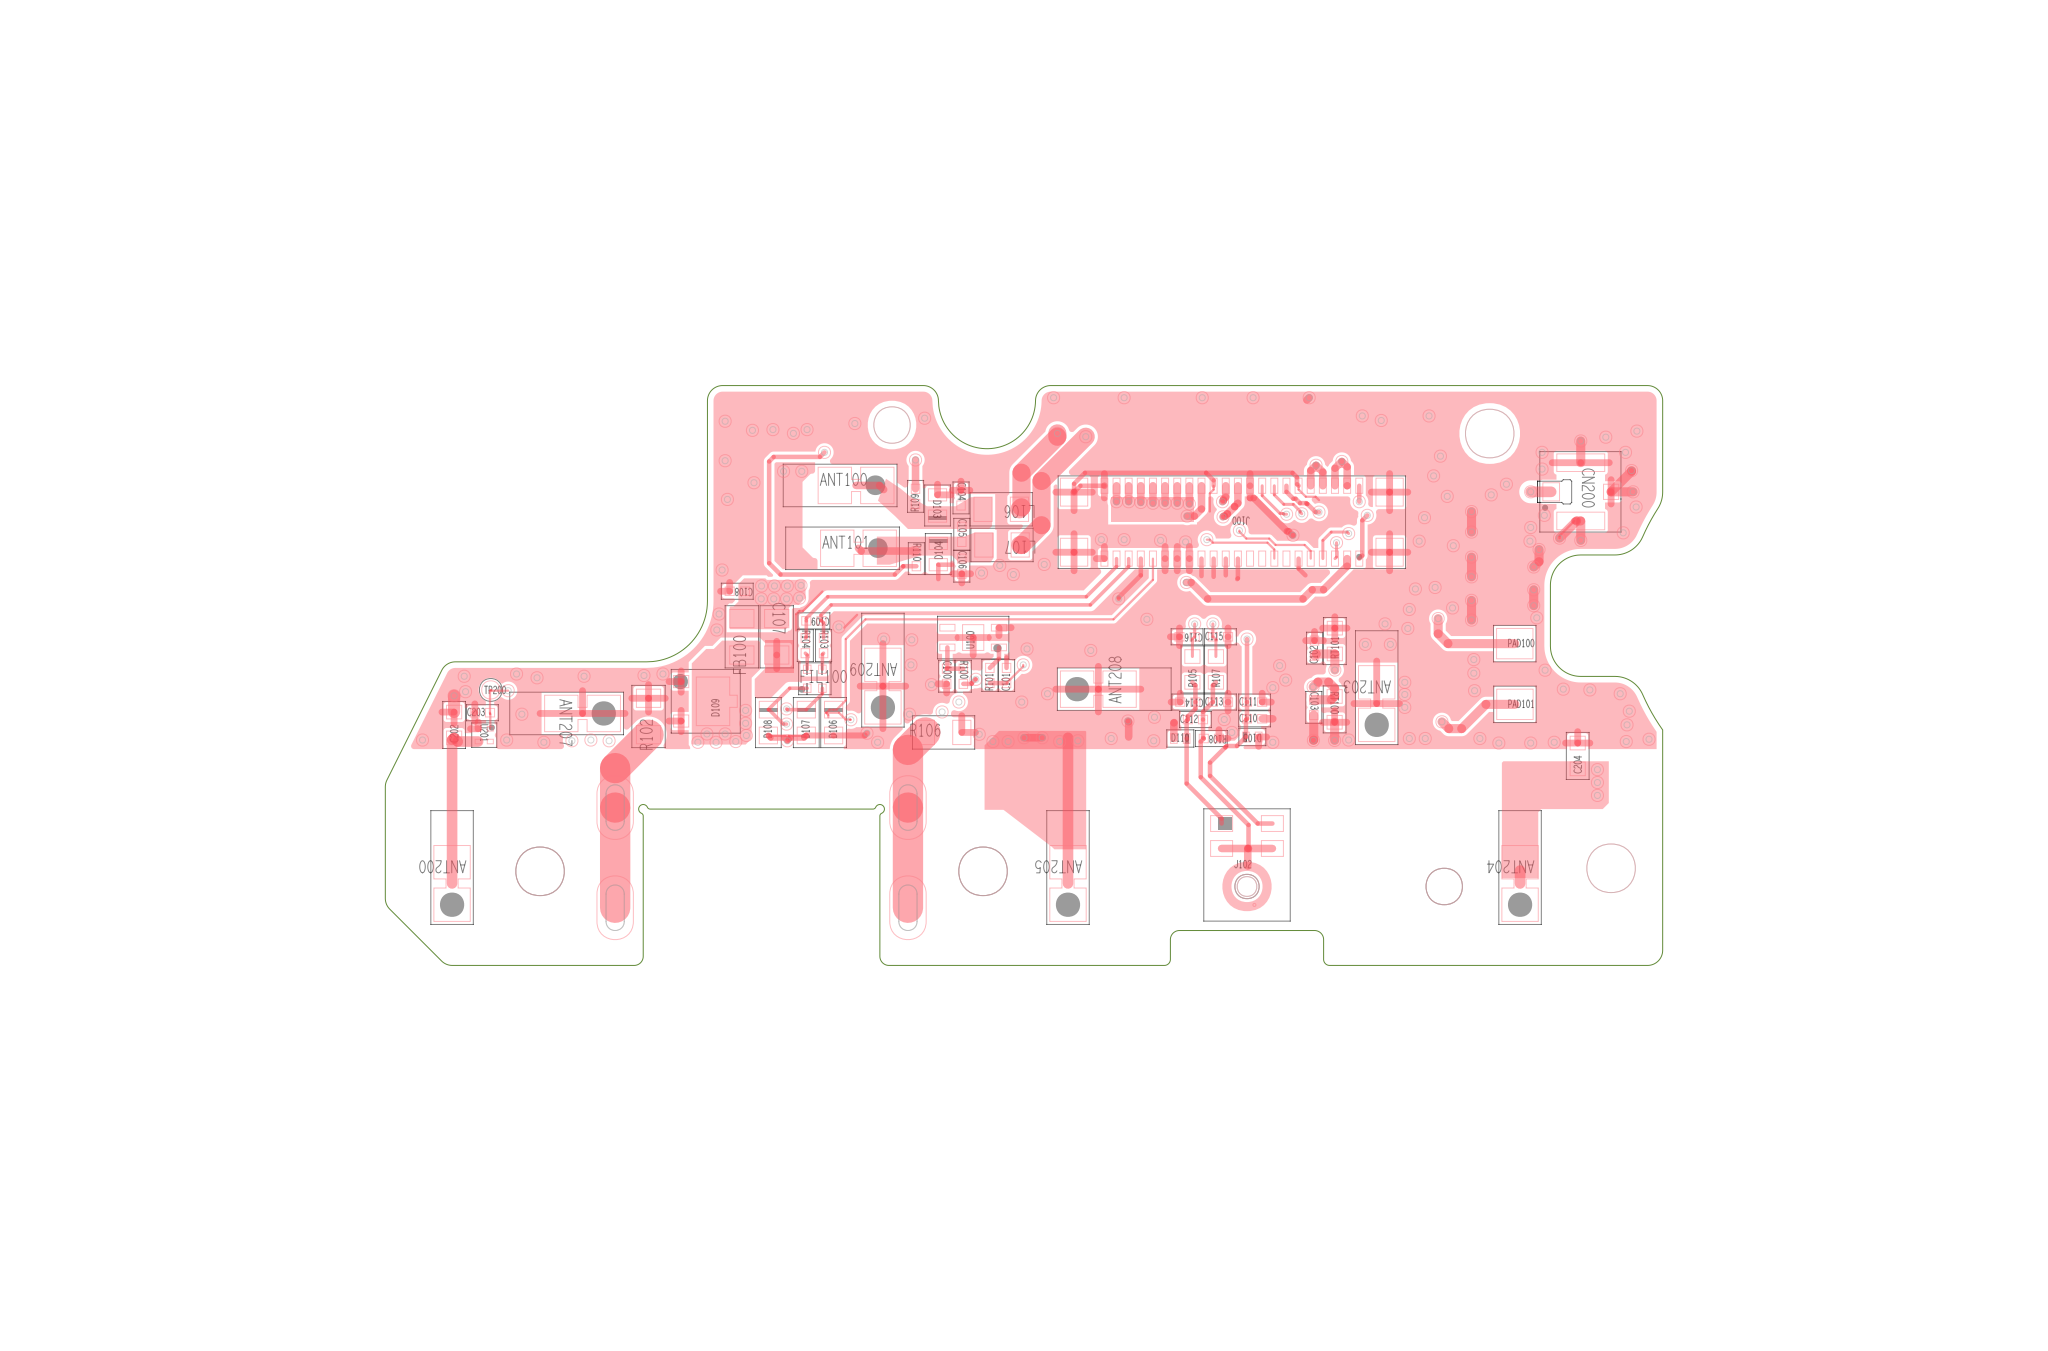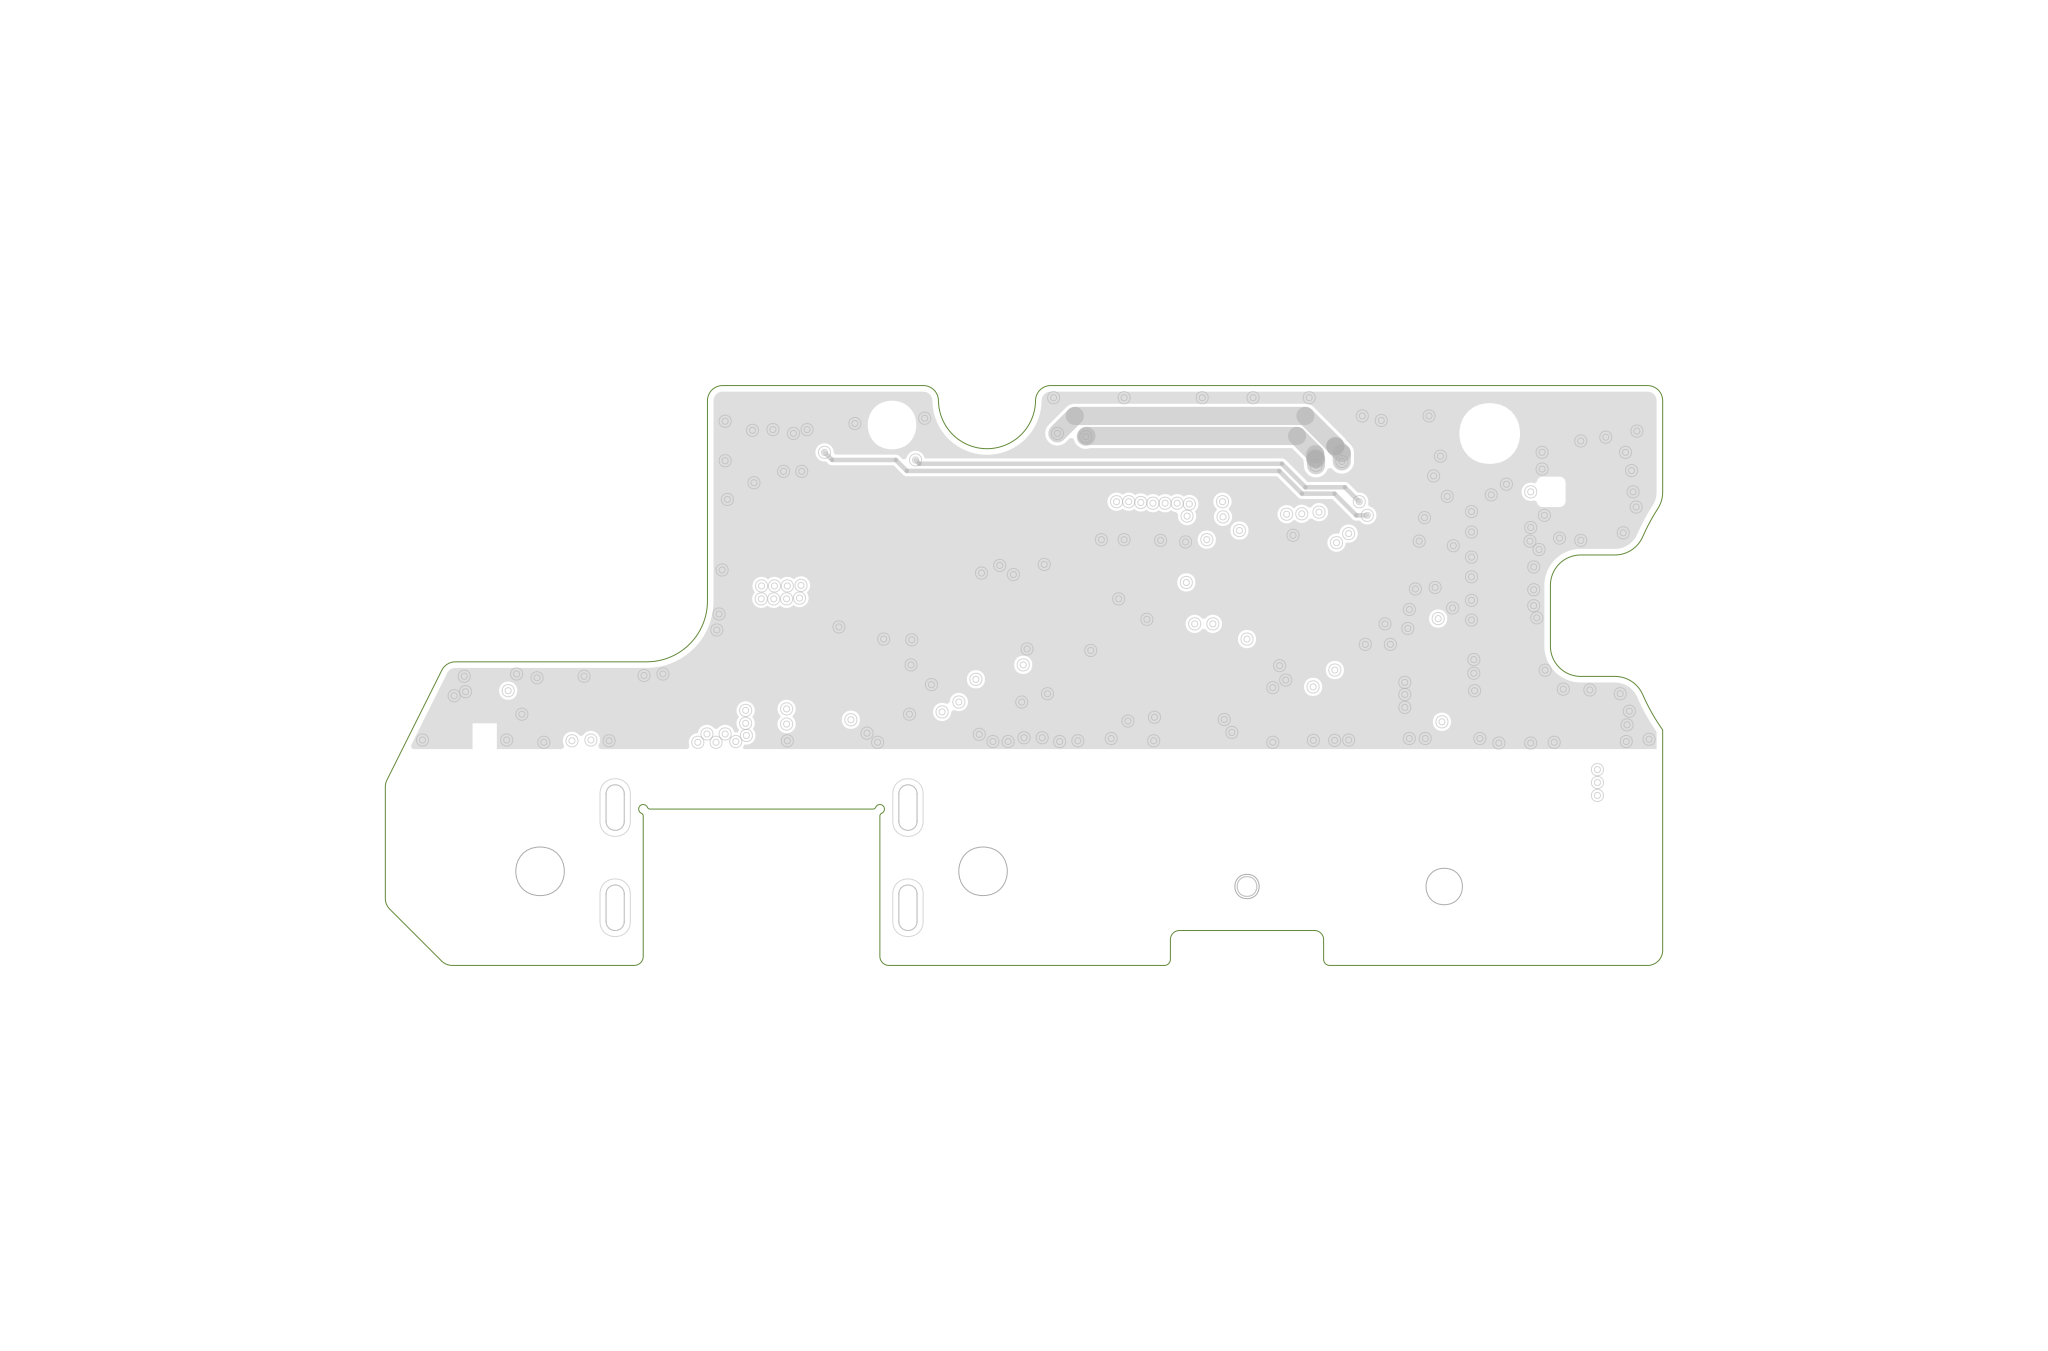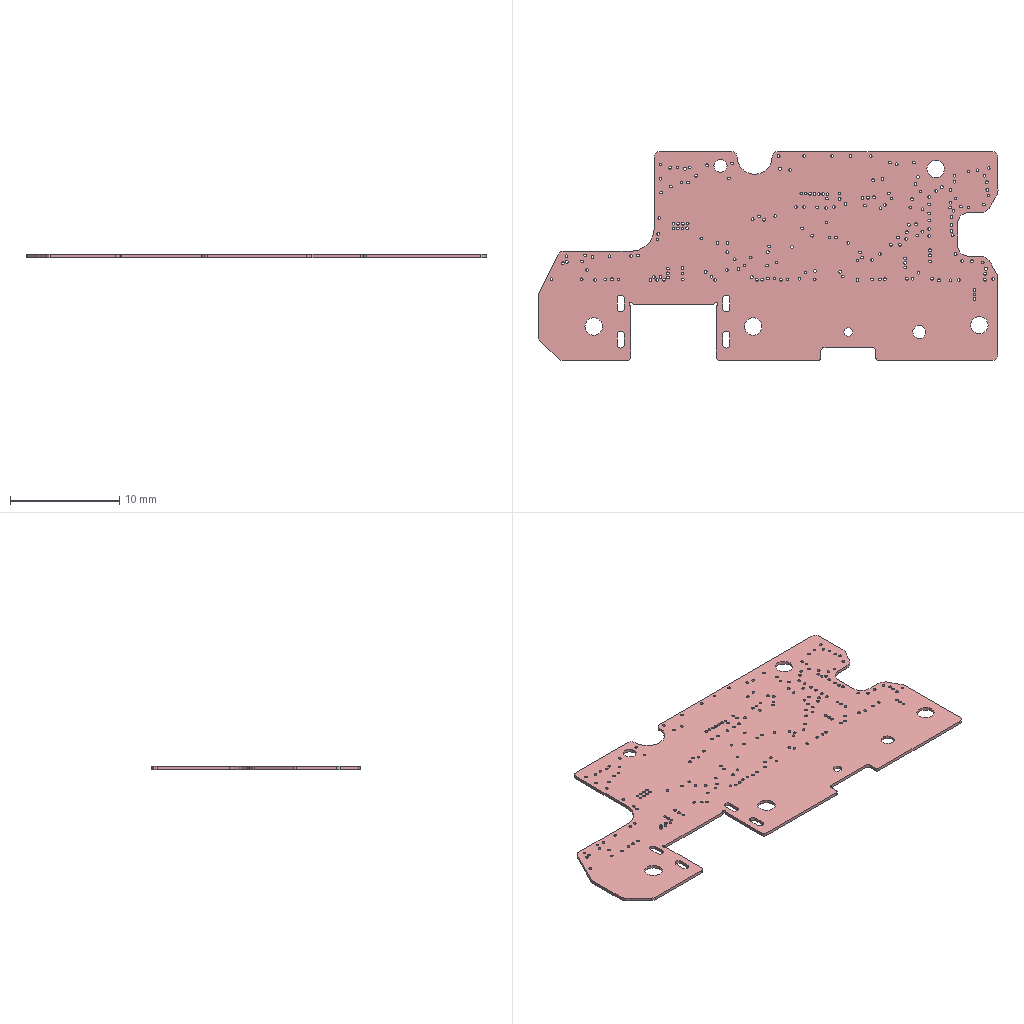Circuit board layout | Cadence Allegro | box 42.1 x 19.1 x 0.3 mm
Layer stack:
# Cadence Allegro layer stack of  (unit mm; from the constraint file cross-section; dielectric type: 0 not recorded (Allegro does not mark core vs prepreg), 3 surface material)
index,name,kind,layer,copper_thickness_mm,dielectric_type,dielectric_thickness_mm,dielectric_material,dielectric_constant
0,Top Surface,other,,,,,,
1,TOP,copper,TOP,0.032,,,,
2,Dielectric1,dielectric,,,0,0.075,FR-4,3.9
3,L2,copper,L2,0.017,,,,
4,Dielectric2,dielectric,,,0,0.1,FR-4,3.9
5,L3,copper,L3,0.017,,,,
6,Dielectric3,dielectric,,,0,0.075,FR-4,3.9
7,BOTTOM,copper,BOTTOM,0.032,,,,
8,Bottom Surface,other,,,,,,
# drill layer pairs: low layer,high layer
drill_pair,TOP,BOTTOM
Part placement:
REFDES,COMP_VALUE,SYM_NAME,SYM_X,SYM_Y,SYM_ROTATE,SYM_MIRROR
ANT100,818001475,PIN_ANT_818001475,36.29,-20.74,0.000,NO
ANT101,818001475,PIN_ANT_818001475,36.37,-22.81,0.000,NO
ANT200,818001103,PIN_ANT_818001103,23.5,-33.275,180.000,NO
ANT203,818001103,PIN_ANT_818001103,53.975,-27.35,180.000,NO
ANT204,818001103,PIN_ANT_818001103,58.7,-33.275,180.000,NO
ANT205,818001103,PIN_ANT_818001103,43.8,-33.275,180.000,NO
ANT207,818001103,PIN_ANT_818001103,27.225,-28.25,270.000,NO
ANT208,818001103,PIN_ANT_818001103,45.375,-27.45,90.000,NO
ANT209,818001103,PIN_ANT_818001103,37.7,-26.775,180.000,NO
C100,100NF,C0201,39.8,-27.025,270.000,NO
C101,100NF,C0201,41.775,-27,90.000,NO
C102,33PF,C0201,51.925,-26.1,90.000,NO
C103,33PF,C0201,51.9,-28.05,270.000,NO
C104,33PF,C0201,40.275,-21.15,270.000,NO
C105,100PF,C0201,40.3,-22.35,270.000,NO
C106,33PF,C0201,40.3,-23.4,270.000,NO
C107,1UF,C0603,34.2,-25.725,270.000,NO
C108,33PF,C0201,32.9,-24.225,180.000,NO
C109,2.2PF,C0201,35.425,-25.2,180.000,NO
C110,33PF,C0201,49.95,-28.425,0.000,NO
C111,100NF,C0201,49.95,-27.875,0.000,NO
C112,33PF,C0201,48,-28.45,0.000,NO
C113,33PF,C0201,48.825,-27.875,0.000,NO
C114,33PF,C0201,47.75,-27.875,180.000,NO
C115,10PF,C0201,48.825,-25.725,0.000,NO
C116,10PF,C0201,47.725,-25.725,180.000,NO
C202,22nH,L0402,23.567,-28.63,90.000,NO
C203,39pF,C0201,24.5,-28.225,0.000,NO
C204,1pF,C0402,60.6,-29.65,90.000,NO
CN200,20449C1,RF_20449C1,60.7,-20.95,270.000,NO
D100,19-217UTD_S3393_TR8,19-217UTD_S3393_TR8,44.7,-31.725,0.000,YES
D101,19-217UTD_S3393_TR8,19-217UTD_S3393_TR8,22.7,-31.725,180.000,YES
D103,PESDNC2FD12VBH,DFN1006-2L,39.5,-21.4,270.000,NO
D104,PESDNC2FD12VBH,DFN1006-2L,39.525,-23,90.000,NO
D105,VESD5451Z-2/TR,DFN0603-2L,49.875,-29.025,180.000,NO
D106,VESD5311N-2/TR,DFN1006-2,36.075,-28.55,90.000,NO
D107,VESD5311N-2/TR,DFN1006-2,35.175,-28.55,90.000,NO
D108,VESD5311N-2/TR,DFN1006-2,33.925,-28.55,90.000,NO
D109,PTVSHC3N15VU,DFN2X2-3L,31.85,-27.85,90.000,NO
D110,VESD5451Z-2/TR,DFN0603-2L,47.5,-29.075,0.000,NO
FB100,0R,R0603,33.05,-25.725,90.000,NO
FIL100,ICMF062P900MFR,EMI4_0P87X0P67X0P62_INNOCHIPS,35.456,-27.107,0.000,NO
J100,AXE544127D_CW,BTB_AXE544124_CW,49.2,-21.95,180.000,NO
J101,3.2.01.0220,USB_3_2_01_0220,33.7,-33,0.000,YES
J102,S18OB381-015,S18OB381-015,49.7,-33.24,0.000,NO
L100,39NH,L0201,44.175,-32.575,180.000,YES
L101,39NH,L0201,45.325,-32.55,0.000,YES
L102,39NH,L0201,23.2,-32.625,0.000,YES
L103,39NH,L0201,22.125,-32.625,0.000,YES
L106,FB MH1608HL121-T,L0603,41.6,-21.525,180.000,NO
L107,FB MH1608HL121-T,L0603,41.625,-22.7,180.000,NO
L200,0R,R0402,60.825,-28.4,180.000,YES
L201,2.7nH,L0402,58.575,-26.675,180.000,YES
PAD100,PAD_R1P0X1P2,PAD_R1P0X1P2,58.525,-25.95,0.000,NO
PAD101,PAD_R1P0X1P2,PAD_R1P0X1P2,58.53,-27.95,0.000,NO
PAD200,K3.1.01.0000,PIN_GND_5M89A463VK,49.99,-20.935,270.000,YES
PAD201,K3.1.01.0000,PIN_GND_5M89A463VK,36.975,-21.45,270.000,YES
PAD202,K3.1.01.0000,PIN_GND_5M89A463VK,36.475,-26.95,270.000,YES
PAD203,K3.1.01.0000,PIN_GND_5M89A463VK,55.975,-26.95,270.000,YES
PAD204,K3.1.01.0000,PIN_GND_5M89A463VK,45.975,-26.95,270.000,YES
R100,0R,R0201,40.35,-27.025,270.000,NO
R101,0R,R0201,41.225,-27,90.000,NO
R102,0R,R0603,29.975,-28.35,90.000,NO
R103,0R,R0201,35.743,-26.015,270.000,NO
R104,0R,R0201,35.143,-26.015,270.000,NO
R105,0R,R0402,47.9,-26.8,90.000,NO
R106,0R,R0603,39.7,-28.875,0.000,NO
R107,0R,R0402,48.675,-26.8,90.000,NO
R108,0R,R0201,48.525,-29.075,180.000,NO
R109,0R,R0201,38.775,-21.1,90.000,NO
R110,0R,R0201,38.803,-23.15,270.000,NO
R200,0R,R0402,58.15,-27.975,90.000,YES
R201,0R,R0402,58.15,-25.35,90.000,YES
R203,0R,R0402,59.3,-27.975,90.000,YES
RT100,AVLC18S02003,R0402,52.588,-28.116,270.000,NO
RT101,AVLC18S02003,R0402,52.595,-25.865,90.000,NO
TP200,TP_c0P6,TP_C0P6,24.775,-27.475,0.000,NO
U100,BU52012NVX-TR,SSON004X1216,40.675,-25.75,90.000,NO
U201,TCP-4118UB-DT,WLCSP4_0P609X0P626X0P445,24.56,-28.965,270.000,NO
Pad and via stacks:
# Allegro (Cadence) via spans and padstacks; design units: ("millimeters" 4 10000)
# via spans: padstack,start_layer,end_layer,net_example,count
VIA02-04-T-B,ETCH/TOP,ETCH/BOTTOM,GND,205
# Allegro padstack definitions: name,start_layer,end_layer,drill,plating,holeType,type
TOP-L2,"ETCH/TOP","ETCH/L2",0.1,"PLATED","circle_drill","bbvia"
L2-L3,"ETCH/L2","ETCH/L3",0.1,"PLATED","circle_drill","bbvia"
0P28X0P3SMD,"ETCH/TOP","ETCH/TOP",0.0,"PLATED","none","smd"
0P24X0P32SMD-OB0P19X0P27PASTE,"ETCH/TOP","ETCH/TOP",0.0,"PLATED","none","smd"
0P5SSMD,"ETCH/TOP","ETCH/TOP",0.0,"PLATED","none","smd"
0P37X0P5SMD,"ETCH/TOP","ETCH/TOP",0.0,"PLATED","none","smd"
0P4X0P7SMD_NP,"ETCH/TOP","ETCH/TOP",0.0,"PLATED","none","smd"
0P4X0P5SMD,"ETCH/TOP","ETCH/TOP",0.0,"PLATED","none","smd"
0P45X0P53SMD,"ETCH/TOP","ETCH/TOP",0.0,"PLATED","none","smd"
0P23X0P65SMD_CONNECTOR,"ETCH/TOP","ETCH/TOP",0.0,"PLATED","none","smd"
0P5X1P6SMD,"ETCH/TOP","ETCH/TOP",0.0,"PLATED","none","smd"
0P55X0P6SMD,"ETCH/TOP","ETCH/TOP",0.0,"PLATED","none","smd"
1P48X2P0SMD-NP,"ETCH/TOP","ETCH/TOP",0.0,"NON_PLATED","none","smd"
0P1CSMD-NSOLDER-NP,"ETCH/TOP","ETCH/TOP",0.0,"PLATED","none","smd"
0P4X1P4SMD,"ETCH/TOP","ETCH/TOP",0.0,"PLATED","none","smd"
0P45X1P4SMD,"ETCH/TOP","ETCH/TOP",0.0,"PLATED","none","smd"
0P45X0P5SMD,"ETCH/TOP","ETCH/TOP",0.0,"PLATED","none","smd"
0P6X0P8SMD,"ETCH/TOP","ETCH/TOP",0.0,"PLATED","none","smd"
0P45XOP95SMD,"ETCH/TOP","ETCH/TOP",0.0,"PLATED","none","smd"
0P35X2P3SMD,"ETCH/TOP","ETCH/TOP",0.0,"PLATED","none","smd"
0P35X1P3SMD,"ETCH/TOP","ETCH/TOP",0.0,"PLATED","none","smd"
2P0CSMD_NP,"ETCH/TOP","ETCH/TOP",0.0,"PLATED","none","smd"
0P1CSMD,"ETCH/TOP","ETCH/TOP",0.0,"PLATED","none","smd"
0P2X0P6SMD,"ETCH/TOP","ETCH/TOP",0.0,"PLATED","none","smd"
0P2X0P4SMD,"ETCH/TOP","ETCH/TOP",0.0,"PLATED","none","smd"
0P2CSMD,"ETCH/TOP","ETCH/TOP",0.0,"PLATED","none","smd"
1P1X1P3SMD,"ETCH/TOP","ETCH/TOP",0.0,"PLATED","none","smd"
1P0CSMD_NP,"ETCH/TOP","ETCH/TOP",0.0,"PLATED","none","smd"
L8-L9,,,0.1,"PLATED","circle_drill","through"
L9-BOTTOM,"ETCH/BOTTOM","ETCH/BOTTOM",0.1,"PLATED","circle_drill","bbvia"
L7-L8,,,0.1,"PLATED","circle_drill","through"
L3-L4,"ETCH/L3","ETCH/L3",0.1,"PLATED","circle_drill","bbvia"
L4-L7,,,0.2,"PLATED","circle_drill","through"
VIA0P1X0P25,"ETCH/TOP","ETCH/BOTTOM",0.1,"PLATED","circle_drill","through"
VIA0P2X0P4,"ETCH/TOP","ETCH/BOTTOM",0.2,"PLATED","circle_drill","through"
L1-L10,"ETCH/TOP","ETCH/BOTTOM",0.2,"PLATED","circle_drill","through"
P0P6X1P7OB1P4X2P9R,"ETCH/TOP","ETCH/BOTTOM",0.6,"PLATED","oval slot","through"
P0P6X1P7OB1P25X2P9R,"ETCH/TOP","ETCH/BOTTOM",0.6,"PLATED","oval slot","through"
NPIN472,"ETCH/TOP","ETCH/BOTTOM",1.2,"NON_PLATED","circle_drill","through"
NPIN630,"ETCH/TOP","ETCH/BOTTOM",1.6,"NON_PLATED","circle_drill","through"
PIN_ANT,"ETCH/TOP","ETCH/TOP",0.0,"PLATED","none","smd"
R0P28X0P3,"ETCH/TOP","ETCH/TOP",0.0,"PLATED","none","smd"
R0P6X0P8,"ETCH/TOP","ETCH/TOP",0.0,"PLATED","none","smd"
R0P45X0P5,"ETCH/TOP","ETCH/TOP",0.0,"PLATED","none","smd"
R0P55X0P6,"ETCH/TOP","ETCH/TOP",0.0,"PLATED","none","smd"
R0P58X1P58,"ETCH/TOP","ETCH/TOP",0.0,"PLATED","none","smd"
SQ0P5,"ETCH/TOP","ETCH/TOP",0.0,"PLATED","none","smd"
R0P4X0P7_PMR0P3X0P6_SMR0P5X0P8,"ETCH/TOP","ETCH/TOP",0.0,"PLATED","none","smd"
R0P24X0P32_PMOB0P19X0P27,"ETCH/TOP","ETCH/TOP",0.0,"PLATED","none","smd"
R0P5X0P6,"ETCH/TOP","ETCH/TOP",0.0,"PLATED","none","smd"
SQ0P3,"ETCH/TOP","ETCH/TOP",0.0,"PLATED","none","smd"
R0P9X0P92,"ETCH/TOP","ETCH/TOP",0.0,"PLATED","none","smd"
R0P23X0P5,"ETCH/TOP","ETCH/TOP",0.0,"PLATED","none","smd"
PTH_OB0P6X1P5OB1P2X2P1,"ETCH/TOP","ETCH/BOTTOM",0.6,"PLATED","oval slot","through"
R0P4X1P05,"ETCH/TOP","ETCH/TOP",0.0,"PLATED","none","smd"
R0P622X1P032,"ETCH/TOP","ETCH/TOP",0.0,"PLATED","none","smd"
R0P5X1P032,"ETCH/TOP","ETCH/TOP",0.0,"PLATED","none","smd"
R0P65X0P7,"ETCH/TOP","ETCH/TOP",0.0,"NON_PLATED","none","smd"
R0P5X2P5,"ETCH/TOP","ETCH/TOP",0.0,"PLATED","none","smd"
R0P8X1P8_NP,"ETCH/TOP","ETCH/TOP",0.0,"PLATED","none","smd"
R0P51X0P61,"ETCH/TOP","ETCH/TOP",0.0,"PLATED","none","smd"
C0P6_NP,"ETCH/TOP","ETCH/TOP",0.0,"PLATED","none","smd"
R0P4X0P55_NP,"ETCH/TOP","ETCH/TOP",0.0,"PLATED","none","smd"
SGP100_P,"ETCH/TOP","ETCH/TOP",0.0,"PLATED","none","smd"
R0P22X0P5,"ETCH/TOP","ETCH/TOP",0.0,"NON_PLATED","none","smd"
R0P7X0P85,"ETCH/TOP","ETCH/TOP",0.0,"PLATED","none","smd"
C0P25_BGA0P4,"ETCH/TOP","ETCH/TOP",0.0,"PLATED","none","smd"
TCP-3127H-DT,"ETCH/TOP","ETCH/TOP",0.0,"PLATED","none","smd"
R0P15X0P43,"ETCH/TOP","ETCH/TOP",0.0,"PLATED","none","smd"
R0P15X0P73,"ETCH/TOP","ETCH/TOP",0.0,"PLATED","none","smd"
VIA02-04-T-B,"ETCH/TOP","ETCH/BOTTOM",0.2,"PLATED","circle_drill","through"
PTH_C1P6C2P0,"ETCH/TOP","ETCH/BOTTOM",1.6,"PLATED","circle_drill","through"
NPTH_C1P6,"ETCH/TOP","ETCH/BOTTOM",1.6,"NON_PLATED","circle_drill","through"
NPTH_C1P2,"ETCH/TOP","ETCH/BOTTOM",1.2,"NON_PLATED","circle_drill","through"
R2P0X3P0_NP,"ETCH/TOP","ETCH/TOP",0.0,"PLATED","none","smd"
R0P4X0P5_PMR0P4X0P5_SMR0P5X0P6,"ETCH/TOP","ETCH/TOP",0.0,"PLATED","none","smd"
DFN2020-3,"ETCH/TOP","ETCH/TOP",0.0,"PLATED","none","smd"
HOLE_C1P6C2P8_SISLEY2,"ETCH/TOP","ETCH/BOTTOM",1.6,"PLATED","circle_drill","through"
R1P48X2P0_NP,"ETCH/TOP","ETCH/TOP",0.0,"NON_PLATED","none","smd"
R1P0X1P2,"ETCH/TOP","ETCH/TOP",0.0,"PLATED","none","smd"
R1P5X3P0_NP,"ETCH/TOP","ETCH/TOP",0.0,"PLATED","none","smd"
R0P522X0P725,"ETCH/TOP","ETCH/TOP",0.0,"PLATED","none","smd"
NPTH_C0P65,"ETCH/TOP","ETCH/BOTTOM",0.65,"NON_PLATED","circle_drill","through"
C0P1,"ETCH/TOP","ETCH/TOP",0.0,"PLATED","none","smd"
R0P4X0P5,"ETCH/TOP","ETCH/TOP",0.0,"PLATED","none","smd"
DFN2X2-3L,"ETCH/TOP","ETCH/TOP",0.0,"PLATED","none","smd"
R0P22X0P32,"ETCH/TOP","ETCH/TOP",0.0,"PLATED","none","smd"
R0P4X0P6,"ETCH/TOP","ETCH/TOP",0.0,"PLATED","none","smd"
R0P25X0P275,"ETCH/TOP","ETCH/TOP",0.0,"PLATED","none","smd"
NPIN315,"ETCH/TOP","ETCH/BOTTOM",0.8,"NON_PLATED","circle_drill","through"
SQ0P8,"ETCH/TOP","ETCH/TOP",0.0,"PLATED","none","smd"
R0P15X0P2_PMR0P15X0P2,"ETCH/TOP","ETCH/TOP",0.0,"PLATED","none","smd"
PIN_ANT_818001105,"ETCH/TOP","ETCH/TOP",0.0,"PLATED","none","smd"
NMTG630,"ETCH/TOP","ETCH/BOTTOM",1.6,"NON_PLATED","circle_drill","through"
NMTG315,"ETCH/TOP","ETCH/BOTTOM",0.8,"NON_PLATED","circle_drill","through"
NMTG472,"ETCH/TOP","ETCH/BOTTOM",1.2,"NON_PLATED","circle_drill","through"
Design rules, without the lines most boards share, first 9 of 32 lines:
# Cadence Allegro design rules of  (from the Constraint Manager export constraints.dcfx, design unit mm; typed fields in mm)
# columns: name | kind | enabled | priority | scope1 | scope2 | descriptor | typed fields (field=value)
# Allegro precedence (priority 1 wins): 1 Region class-to-class, 2 Region class, 3 Region, 4 class-to-class, 5 DiffPair/Bus/NetGroup override, 6 NetClass, 7 constraint set (CSet) default
# per-layer values are written LAYER=value in the descriptor and LAYER:mm in the typed field; a maximum of 0 means no limit set
# --- net classes (and buses / net groups) ---
# (no net classes defined: every net uses the default constraint sets)
# --- track widths, neck and differential-pair gap (physical constraint sets) ---
50O | PhysicalCSet | enabled | 7 | Net(3): N18809773, N18731084, N18730979 | All | Physical Constraint (Min Line Width=0.353mm) (Max Line Width=5mm) (Min Neck Width=0.075mm) (Max Neck Length=1mm) (DiffPair Primary Gap=0mm) (DiffPair Neck Gap=0mm) (DiffPair Min Space=0mm) (DiffPair Coupled +Tol=0mm) (DiffPair Coupled -Tol=0mm) (Min BB Via Stagger=0mm) (Max BB Via Stagger=0mm) (T-junctions=ANYWHERE) (Pad-pad direct connect=TOP:VIAS_PINS_ONLY,L2:NOT_ALLOWED,L3:VIAS_PINS_ONLY,BOTTOM:VIAS_PINS_ONLY) (Allowed vias=VIA02-04-T-B) | min_line_width=0.353 min_neck_width=0.075 min_bvia_stagger=0 max_bvia_stagger=0 ts_allowed=ANYWHERE diffp_primary_gap=0 diffp_neck_gap=0 max_line_width=5 maximum_neck_length=1 pad_pad_direct_connect=TOP:VIAS_PINS_ONLY,L2:NOT_ALLOWED,L3:VIAS_PINS_ONLY,BOTTOM:VIAS_PINS_ONLY allow_on_etch_subclass=TRUE diffp_coupled_plus=0 diffp_coupled_minus=0 diffp_min_space=0 vias=VIA02-04-T-B
DIFF 90OM | PhysicalCSet | enabled | 7 | Net(6): N18858337, N18858369, N18858335, N18858430, USB_HS_D_P, USB_HS_D_M | All | Physical Constraint (Min Line Width=0.119mm) (Max Line Width=5mm) (Min Neck Width=0.05mm) (Max Neck Length=1mm) (DiffPair Primary Gap=0.15mm) (DiffPair Neck Gap=0.15mm) (DiffPair Min Space=0mm) (DiffPair Coupled +Tol=0mm) (DiffPair Coupled -Tol=0mm) (Min BB Via Stagger=0mm) (Max BB Via Stagger=0mm) (T-junctions=ANYWHERE) (Pad-pad direct connect=TOP:VIAS_PINS_ONLY,L2:NOT_ALLOWED,L3:VIAS_PINS_ONLY,BOTTOM:VIAS_PINS_ONLY) (Allowed vias=VIA02-04-T-B) | min_line_width=0.119 min_neck_width=0.05 min_bvia_stagger=0 max_bvia_stagger=0 ts_allowed=ANYWHERE diffp_primary_gap=0.15 diffp_neck_gap=0.15 max_line_width=5 maximum_neck_length=1 pad_pad_direct_connect=TOP:VIAS_PINS_ONLY,L2:NOT_ALLOWED,L3:VIAS_PINS_ONLY,BOTTOM:VIAS_PINS_ONLY allow_on_etch_subclass=TRUE diffp_coupled_plus=0 diffp_coupled_minus=0 diffp_min_space=0 vias=VIA02-04-T-B